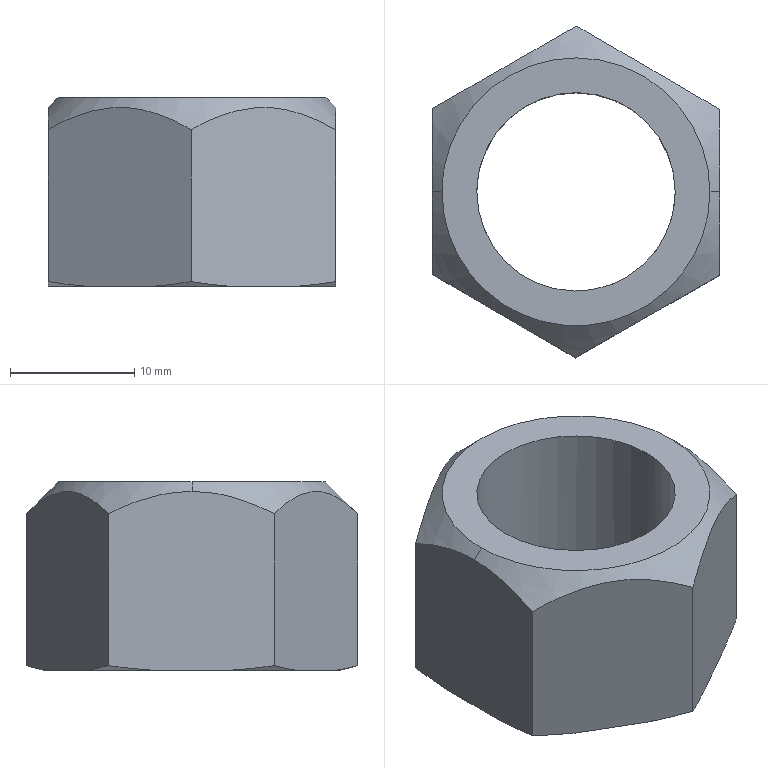Part | STEP file | GB/T6184-20001 type all-metal hex lock nut M16 | 1 solid | 20 faces | box 23.219 x 26.75 x 15.2 mm | volume 3899 mm3 | cone 10 | plane 8 | cylinder 2 | commonest cylinder face diameters 16 x2
STEP:
#1=CARTESIAN_POINT('',(-10.8,0.,15.2));
#2=VERTEX_POINT('',#1);
#3=CARTESIAN_POINT('',(10.8,0.,15.2));
#4=VERTEX_POINT('',#3);
#5=CARTESIAN_POINT('',(0.,0.,15.2));
#6=DIRECTION('',(0.,0.,-1.));
#7=AXIS2_PLACEMENT_3D('',#5,#6,$);
#8=CIRCLE('',#7,10.8);
#9=EDGE_CURVE('',#2,#4,#8,.F.);
#10=ORIENTED_EDGE('',*,*,#9,.F.);
#11=CARTESIAN_POINT('',(-11.583,0.,14.417));
#12=VERTEX_POINT('',#11);
#13=CARTESIAN_POINT('',(-353558.791,0.,-353532.791));
#14=DIRECTION('',(-0.7071,0.,-0.7071));
#15=VECTOR('',#14,1.);
#16=LINE('',#13,#15);
#17=EDGE_CURVE('',#2,#12,#16,.T.);
#18=ORIENTED_EDGE('',*,*,#17,.T.);
#19=CARTESIAN_POINT('',(-11.597,-3.411,13.912));
#20=VERTEX_POINT('',#19);
#21=CARTESIAN_POINT('',(-11.583,0.,14.417));
#22=CARTESIAN_POINT('',(-11.586,-0.8291,14.414));
#23=CARTESIAN_POINT('',(-11.59,-1.659,14.33));
#24=CARTESIAN_POINT('',(-11.593,-2.511,14.17));
#25=CARTESIAN_POINT('',(-11.597,-3.411,13.912));
#26=B_SPLINE_CURVE_WITH_KNOTS('',4,(#21,#22,#23,#24,#25),.UNSPECIFIED.,.F.,.U.,(5,5),(0.,28.825),.UNSPECIFIED.);
#27=EDGE_CURVE('',#12,#20,#26,.T.);
#28=ORIENTED_EDGE('',*,*,#27,.T.);
#29=CARTESIAN_POINT('',(-11.609,-6.642,12.625));
#30=VERTEX_POINT('',#29);
#31=CARTESIAN_POINT('',(-11.597,-3.411,13.912));
#32=CARTESIAN_POINT('',(-11.6,-4.397,13.63));
#33=CARTESIAN_POINT('',(-11.605,-5.447,13.222));
#34=CARTESIAN_POINT('',(-11.609,-6.642,12.625));
#35=B_SPLINE_CURVE_WITH_KNOTS('',3,(#31,#32,#33,#34),.UNSPECIFIED.,.F.,.U.,(4,4),(0.,23.689),.UNSPECIFIED.);
#36=EDGE_CURVE('',#20,#30,#35,.T.);
#37=ORIENTED_EDGE('',*,*,#36,.T.);
#38=CARTESIAN_POINT('',(-2.874,-11.731,13.922));
#39=VERTEX_POINT('',#38);
#40=CARTESIAN_POINT('',(-11.609,-6.642,12.625));
#41=CARTESIAN_POINT('',(-9.468,-7.889,13.864));
#42=CARTESIAN_POINT('',(-7.794,-8.865,14.408));
#43=CARTESIAN_POINT('',(-6.199,-9.794,14.622));
#44=CARTESIAN_POINT('',(-4.639,-10.703,14.5));
#45=CARTESIAN_POINT('',(-2.874,-11.731,13.922));
#46=B_SPLINE_CURVE_WITH_KNOTS('',5,(#40,#41,#42,#43,#44,#45),.UNSPECIFIED.,.F.,.U.,(6,6),(0.,81.885),.UNSPECIFIED.);
#47=EDGE_CURVE('',#30,#39,#46,.T.);
#48=ORIENTED_EDGE('',*,*,#47,.T.);
#49=CARTESIAN_POINT('',(-0.05261,-13.375,12.625));
#50=VERTEX_POINT('',#49);
#51=CARTESIAN_POINT('',(-2.874,-11.731,13.922));
#52=CARTESIAN_POINT('',(-2.013,-12.233,13.64));
#53=CARTESIAN_POINT('',(-1.097,-12.766,13.229));
#54=CARTESIAN_POINT('',(-0.05261,-13.375,12.625));
#55=B_SPLINE_CURVE_WITH_KNOTS('',3,(#51,#52,#53,#54),.UNSPECIFIED.,.F.,.U.,(4,4),(0.,23.96),.UNSPECIFIED.);
#56=EDGE_CURVE('',#39,#50,#55,.T.);
#57=ORIENTED_EDGE('',*,*,#56,.T.);
#58=CARTESIAN_POINT('',(8.723,-8.355,13.922));
#59=VERTEX_POINT('',#58);
#60=CARTESIAN_POINT('',(-0.05261,-13.375,12.625));
#61=CARTESIAN_POINT('',(2.098,-12.144,13.864));
#62=CARTESIAN_POINT('',(3.78,-11.182,14.408));
#63=CARTESIAN_POINT('',(5.382,-10.266,14.622));
#64=CARTESIAN_POINT('',(6.95,-9.369,14.5));
#65=CARTESIAN_POINT('',(8.723,-8.355,13.922));
#66=B_SPLINE_CURVE_WITH_KNOTS('',5,(#60,#61,#62,#63,#64,#65),.UNSPECIFIED.,.F.,.U.,(6,6),(0.,81.885),.UNSPECIFIED.);
#67=EDGE_CURVE('',#50,#59,#66,.T.);
#68=ORIENTED_EDGE('',*,*,#67,.T.);
#69=CARTESIAN_POINT('',(11.557,-6.733,12.625));
#70=VERTEX_POINT('',#69);
#71=CARTESIAN_POINT('',(8.723,-8.355,13.922));
#72=CARTESIAN_POINT('',(9.587,-7.86,13.64));
#73=CARTESIAN_POINT('',(10.508,-7.333,13.229));
#74=CARTESIAN_POINT('',(11.557,-6.733,12.625));
#75=B_SPLINE_CURVE_WITH_KNOTS('',3,(#71,#72,#73,#74),.UNSPECIFIED.,.F.,.U.,(4,4),(0.,23.96),.UNSPECIFIED.);
#76=EDGE_CURVE('',#59,#70,#75,.T.);
#77=ORIENTED_EDGE('',*,*,#76,.T.);
#78=CARTESIAN_POINT('',(11.583,0.,14.417));
#79=VERTEX_POINT('',#78);
#80=CARTESIAN_POINT('',(11.557,-6.733,12.625));
#81=CARTESIAN_POINT('',(11.563,-5.119,13.432));
#82=CARTESIAN_POINT('',(11.568,-3.735,13.942));
#83=CARTESIAN_POINT('',(11.574,-2.453,14.264));
#84=CARTESIAN_POINT('',(11.578,-1.227,14.422));
#85=CARTESIAN_POINT('',(11.583,0.,14.417));
#86=B_SPLINE_CURVE_WITH_KNOTS('',5,(#80,#81,#82,#83,#84,#85),.UNSPECIFIED.,.F.,.U.,(6,6),(0.,53.326),.UNSPECIFIED.);
#87=EDGE_CURVE('',#70,#79,#86,.T.);
#88=ORIENTED_EDGE('',*,*,#87,.T.);
#89=CARTESIAN_POINT('',(353558.791,0.,-353532.791));
#90=DIRECTION('',(0.7071,0.,-0.7071));
#91=VECTOR('',#90,1.);
#92=LINE('',#89,#91);
#93=EDGE_CURVE('',#4,#79,#92,.T.);
#94=ORIENTED_EDGE('',*,*,#93,.F.);
#95=EDGE_LOOP('',(#10,#18,#28,#37,#48,#57,#68,#77,#88,#94));
#96=FACE_OUTER_BOUND('',#95,.T.);
#97=CARTESIAN_POINT('',(0.,0.,15.2));
#98=DIRECTION('',(0.,0.,-1.));
#99=DIRECTION('',(1.,0.,0.));
#100=AXIS2_PLACEMENT_3D('',#97,#98,#99);
#101=CONICAL_SURFACE('',#100,10.8,0.7854);
#102=ADVANCED_FACE('',(#96),#101,.T.);
#103=CARTESIAN_POINT('',(10.8,0.,15.2));
#104=CARTESIAN_POINT('',(10.8,1.127,15.2));
#105=CARTESIAN_POINT('',(10.653,2.254,15.2));
#106=CARTESIAN_POINT('',(10.359,3.355,15.2));
#107=CARTESIAN_POINT('',(9.49,5.456,15.2));
#108=CARTESIAN_POINT('',(8.112,7.263,15.2));
#109=CARTESIAN_POINT('',(7.308,8.072,15.2));
#110=CARTESIAN_POINT('',(5.509,9.46,15.2));
#111=CARTESIAN_POINT('',(3.413,10.34,15.2));
#112=CARTESIAN_POINT('',(2.313,10.64,15.2));
#113=CARTESIAN_POINT('',(0.06074,10.947,15.2));
#114=CARTESIAN_POINT('',(-2.195,10.665,15.2));
#115=CARTESIAN_POINT('',(-3.298,10.377,15.2));
#116=CARTESIAN_POINT('',(-5.403,9.521,15.2));
#117=CARTESIAN_POINT('',(-7.218,8.152,15.2));
#118=CARTESIAN_POINT('',(-8.031,7.353,15.2));
#119=CARTESIAN_POINT('',(-9.429,5.561,15.2));
#120=CARTESIAN_POINT('',(-10.321,3.47,15.2));
#121=CARTESIAN_POINT('',(-10.627,2.372,15.2));
#122=CARTESIAN_POINT('',(-10.79,1.223,15.2));
#123=CARTESIAN_POINT('',(-10.8,0.07191,15.2));
#124=CARTESIAN_POINT('',(-10.8,0.04794,15.2));
#125=CARTESIAN_POINT('',(-10.8,0.02397,15.2));
#126=CARTESIAN_POINT('',(-10.8,0.,15.2));
#127=B_SPLINE_CURVE_WITH_KNOTS('',5,(#103,#104,#105,#106,#107,#108,#109,#110,#111,#112,#113,#114,#115,#116,#117,#118,#119,#120,#121,#122,#123,#124,#125,#126),.UNSPECIFIED.,.F.,.U.,(6,3,3,3,3,3,3,6),(0.,7.969,15.938,23.906,31.875,39.844,47.813,47.982),.UNSPECIFIED.);
#128=EDGE_CURVE('',#4,#2,#127,.T.);
#129=ORIENTED_EDGE('',*,*,#128,.T.);
#130=ORIENTED_EDGE('',*,*,#9,.T.);
#131=EDGE_LOOP('',(#129,#130));
#132=FACE_OUTER_BOUND('',#131,.T.);
#133=CARTESIAN_POINT('',(-8.,0.,15.2));
#134=VERTEX_POINT('',#133);
#135=CARTESIAN_POINT('',(8.,0.,15.2));
#136=VERTEX_POINT('',#135);
#137=CARTESIAN_POINT('',(-8.,0.,15.2));
#138=CARTESIAN_POINT('',(-8.,-0.8314,15.2));
#139=CARTESIAN_POINT('',(-7.892,-1.663,15.2));
#140=CARTESIAN_POINT('',(-7.676,-2.475,15.2));
#141=CARTESIAN_POINT('',(-7.038,-4.026,15.2));
#142=CARTESIAN_POINT('',(-6.025,-5.362,15.2));
#143=CARTESIAN_POINT('',(-5.434,-5.96,15.2));
#144=CARTESIAN_POINT('',(-4.11,-6.989,15.2));
#145=CARTESIAN_POINT('',(-2.567,-7.646,15.2));
#146=CARTESIAN_POINT('',(-1.757,-7.872,15.2));
#147=CARTESIAN_POINT('',(-0.09689,-8.107,15.2));
#148=CARTESIAN_POINT('',(1.568,-7.911,15.2));
#149=CARTESIAN_POINT('',(2.384,-7.705,15.2));
#150=CARTESIAN_POINT('',(3.942,-7.085,15.2));
#151=CARTESIAN_POINT('',(5.29,-6.088,15.2));
#152=CARTESIAN_POINT('',(5.895,-5.504,15.2));
#153=CARTESIAN_POINT('',(6.94,-4.193,15.2));
#154=CARTESIAN_POINT('',(7.615,-2.658,15.2));
#155=CARTESIAN_POINT('',(7.85,-1.851,15.2));
#156=CARTESIAN_POINT('',(7.984,-0.9842,15.2));
#157=CARTESIAN_POINT('',(7.999,-0.1147,15.2));
#158=CARTESIAN_POINT('',(8.,-0.07648,15.2));
#159=CARTESIAN_POINT('',(8.,-0.03824,15.2));
#160=CARTESIAN_POINT('',(8.,0.,15.2));
#161=B_SPLINE_CURVE_WITH_KNOTS('',5,(#137,#138,#139,#140,#141,#142,#143,#144,#145,#146,#147,#148,#149,#150,#151,#152,#153,#154,#155,#156,#157,#158,#159,#160),.UNSPECIFIED.,.F.,.U.,(6,3,3,3,3,3,3,6),(0.,5.879,11.757,17.636,23.515,29.393,35.272,35.543),.UNSPECIFIED.);
#162=EDGE_CURVE('',#134,#136,#161,.T.);
#163=ORIENTED_EDGE('',*,*,#162,.F.);
#164=CARTESIAN_POINT('',(8.,0.,15.2));
#165=CARTESIAN_POINT('',(8.,0.8314,15.2));
#166=CARTESIAN_POINT('',(7.892,1.663,15.2));
#167=CARTESIAN_POINT('',(7.676,2.475,15.2));
#168=CARTESIAN_POINT('',(7.038,4.026,15.2));
#169=CARTESIAN_POINT('',(6.025,5.362,15.2));
#170=CARTESIAN_POINT('',(5.434,5.96,15.2));
#171=CARTESIAN_POINT('',(4.11,6.989,15.2));
#172=CARTESIAN_POINT('',(2.567,7.646,15.2));
#173=CARTESIAN_POINT('',(1.757,7.872,15.2));
#174=CARTESIAN_POINT('',(0.09689,8.107,15.2));
#175=CARTESIAN_POINT('',(-1.568,7.911,15.2));
#176=CARTESIAN_POINT('',(-2.384,7.705,15.2));
#177=CARTESIAN_POINT('',(-3.942,7.085,15.2));
#178=CARTESIAN_POINT('',(-5.29,6.088,15.2));
#179=CARTESIAN_POINT('',(-5.895,5.504,15.2));
#180=CARTESIAN_POINT('',(-6.94,4.193,15.2));
#181=CARTESIAN_POINT('',(-7.615,2.658,15.2));
#182=CARTESIAN_POINT('',(-7.85,1.851,15.2));
#183=CARTESIAN_POINT('',(-7.984,0.9842,15.2));
#184=CARTESIAN_POINT('',(-7.999,0.1147,15.2));
#185=CARTESIAN_POINT('',(-8.,0.07648,15.2));
#186=CARTESIAN_POINT('',(-8.,0.03824,15.2));
#187=CARTESIAN_POINT('',(-8.,0.,15.2));
#188=B_SPLINE_CURVE_WITH_KNOTS('',5,(#164,#165,#166,#167,#168,#169,#170,#171,#172,#173,#174,#175,#176,#177,#178,#179,#180,#181,#182,#183,#184,#185,#186,#187),.UNSPECIFIED.,.F.,.U.,(6,3,3,3,3,3,3,6),(0.,5.879,11.757,17.636,23.515,29.393,35.272,35.543),.UNSPECIFIED.);
#189=EDGE_CURVE('',#136,#134,#188,.T.);
#190=ORIENTED_EDGE('',*,*,#189,.F.);
#191=EDGE_LOOP('',(#163,#190));
#192=FACE_BOUND('',#191,.T.);
#193=CARTESIAN_POINT('',(23.166,-0.09113,15.2));
#194=DIRECTION('',(0.,0.,-1.));
#195=DIRECTION('',(-1.,0.,0.));
#196=AXIS2_PLACEMENT_3D('',#193,#194,#195);
#197=PLANE('',#196);
#198=ADVANCED_FACE('',(#132,#192),#197,.F.);
#199=ORIENTED_EDGE('',*,*,#17,.F.);
#200=ORIENTED_EDGE('',*,*,#128,.F.);
#201=ORIENTED_EDGE('',*,*,#93,.T.);
#202=CARTESIAN_POINT('',(11.597,3.411,13.912));
#203=VERTEX_POINT('',#202);
#204=CARTESIAN_POINT('',(11.583,0.,14.417));
#205=CARTESIAN_POINT('',(11.586,0.8291,14.414));
#206=CARTESIAN_POINT('',(11.59,1.659,14.33));
#207=CARTESIAN_POINT('',(11.593,2.511,14.17));
#208=CARTESIAN_POINT('',(11.597,3.411,13.912));
#209=B_SPLINE_CURVE_WITH_KNOTS('',4,(#204,#205,#206,#207,#208),.UNSPECIFIED.,.F.,.U.,(5,5),(0.,28.825),.UNSPECIFIED.);
#210=EDGE_CURVE('',#79,#203,#209,.T.);
#211=ORIENTED_EDGE('',*,*,#210,.T.);
#212=CARTESIAN_POINT('',(11.609,6.642,12.625));
#213=VERTEX_POINT('',#212);
#214=CARTESIAN_POINT('',(11.597,3.411,13.912));
#215=CARTESIAN_POINT('',(11.6,4.397,13.63));
#216=CARTESIAN_POINT('',(11.605,5.447,13.222));
#217=CARTESIAN_POINT('',(11.609,6.642,12.625));
#218=B_SPLINE_CURVE_WITH_KNOTS('',3,(#214,#215,#216,#217),.UNSPECIFIED.,.F.,.U.,(4,4),(0.,23.689),.UNSPECIFIED.);
#219=EDGE_CURVE('',#203,#213,#218,.T.);
#220=ORIENTED_EDGE('',*,*,#219,.T.);
#221=CARTESIAN_POINT('',(2.874,11.731,13.922));
#222=VERTEX_POINT('',#221);
#223=CARTESIAN_POINT('',(11.609,6.642,12.625));
#224=CARTESIAN_POINT('',(9.468,7.889,13.864));
#225=CARTESIAN_POINT('',(7.794,8.865,14.408));
#226=CARTESIAN_POINT('',(6.199,9.794,14.622));
#227=CARTESIAN_POINT('',(4.639,10.703,14.5));
#228=CARTESIAN_POINT('',(2.874,11.731,13.922));
#229=B_SPLINE_CURVE_WITH_KNOTS('',5,(#223,#224,#225,#226,#227,#228),.UNSPECIFIED.,.F.,.U.,(6,6),(0.,81.885),.UNSPECIFIED.);
#230=EDGE_CURVE('',#213,#222,#229,.T.);
#231=ORIENTED_EDGE('',*,*,#230,.T.);
#232=CARTESIAN_POINT('',(0.05261,13.375,12.625));
#233=VERTEX_POINT('',#232);
#234=CARTESIAN_POINT('',(2.874,11.731,13.922));
#235=CARTESIAN_POINT('',(2.013,12.233,13.64));
#236=CARTESIAN_POINT('',(1.097,12.766,13.229));
#237=CARTESIAN_POINT('',(0.05261,13.375,12.625));
#238=B_SPLINE_CURVE_WITH_KNOTS('',3,(#234,#235,#236,#237),.UNSPECIFIED.,.F.,.U.,(4,4),(0.,23.96),.UNSPECIFIED.);
#239=EDGE_CURVE('',#222,#233,#238,.T.);
#240=ORIENTED_EDGE('',*,*,#239,.T.);
#241=CARTESIAN_POINT('',(-8.722,8.355,13.922));
#242=VERTEX_POINT('',#241);
#243=CARTESIAN_POINT('',(0.05261,13.375,12.625));
#244=CARTESIAN_POINT('',(-2.098,12.144,13.864));
#245=CARTESIAN_POINT('',(-3.78,11.182,14.408));
#246=CARTESIAN_POINT('',(-5.382,10.266,14.622));
#247=CARTESIAN_POINT('',(-6.95,9.369,14.5));
#248=CARTESIAN_POINT('',(-8.723,8.355,13.922));
#249=B_SPLINE_CURVE_WITH_KNOTS('',5,(#243,#244,#245,#246,#247,#248),.UNSPECIFIED.,.F.,.U.,(6,6),(0.,81.885),.UNSPECIFIED.);
#250=EDGE_CURVE('',#233,#242,#249,.T.);
#251=ORIENTED_EDGE('',*,*,#250,.T.);
#252=CARTESIAN_POINT('',(-11.557,6.733,12.625));
#253=VERTEX_POINT('',#252);
#254=CARTESIAN_POINT('',(-8.723,8.355,13.922));
#255=CARTESIAN_POINT('',(-9.587,7.86,13.64));
#256=CARTESIAN_POINT('',(-10.508,7.333,13.229));
#257=CARTESIAN_POINT('',(-11.557,6.733,12.625));
#258=B_SPLINE_CURVE_WITH_KNOTS('',3,(#254,#255,#256,#257),.UNSPECIFIED.,.F.,.U.,(4,4),(0.,23.96),.UNSPECIFIED.);
#259=EDGE_CURVE('',#242,#253,#258,.T.);
#260=ORIENTED_EDGE('',*,*,#259,.T.);
#261=CARTESIAN_POINT('',(-11.557,6.733,12.625));
#262=CARTESIAN_POINT('',(-11.563,5.119,13.432));
#263=CARTESIAN_POINT('',(-11.568,3.735,13.942));
#264=CARTESIAN_POINT('',(-11.574,2.453,14.264));
#265=CARTESIAN_POINT('',(-11.578,1.227,14.422));
#266=CARTESIAN_POINT('',(-11.583,0.,14.417));
#267=B_SPLINE_CURVE_WITH_KNOTS('',5,(#261,#262,#263,#264,#265,#266),.UNSPECIFIED.,.F.,.U.,(6,6),(0.,53.326),.UNSPECIFIED.);
#268=EDGE_CURVE('',#253,#12,#267,.T.);
#269=ORIENTED_EDGE('',*,*,#268,.T.);
#270=EDGE_LOOP('',(#199,#200,#201,#211,#220,#231,#240,#251,#260,#269));
#271=FACE_OUTER_BOUND('',#270,.T.);
#272=CARTESIAN_POINT('',(0.,0.,15.2));
#273=DIRECTION('',(0.,0.,-1.));
#274=DIRECTION('',(-1.,0.,0.));
#275=AXIS2_PLACEMENT_3D('',#272,#273,#274);
#276=CONICAL_SURFACE('',#275,10.8,0.7854);
#277=ADVANCED_FACE('',(#271),#276,.T.);
#278=ORIENTED_EDGE('',*,*,#268,.F.);
#279=CARTESIAN_POINT('',(-11.557,6.733,0.3684));
#280=VERTEX_POINT('',#279);
#281=CARTESIAN_POINT('',(-11.557,6.733,6.497));
#282=DIRECTION('',(0.,0.,-1.));
#283=VECTOR('',#282,1.);
#284=LINE('',#281,#283);
#285=EDGE_CURVE('',#253,#280,#284,.T.);
#286=ORIENTED_EDGE('',*,*,#285,.T.);
#287=CARTESIAN_POINT('',(-11.571,3.181,0.000000001));
#288=VERTEX_POINT('',#287);
#289=CARTESIAN_POINT('',(-11.571,3.181,0.000000001));
#290=CARTESIAN_POINT('',(-11.568,3.752,0.03994));
#291=CARTESIAN_POINT('',(-11.566,4.322,0.08839));
#292=CARTESIAN_POINT('',(-11.564,4.89,0.1444));
#293=CARTESIAN_POINT('',(-11.561,5.6,0.2236));
#294=CARTESIAN_POINT('',(-11.558,6.309,0.3127));
#295=CARTESIAN_POINT('',(-11.558,6.45,0.3309));
#296=CARTESIAN_POINT('',(-11.557,6.592,0.3495));
#297=CARTESIAN_POINT('',(-11.557,6.733,0.3684));
#298=B_SPLINE_CURVE_WITH_KNOTS('',5,(#289,#290,#291,#292,#293,#294,#295,#296,#297),.UNSPECIFIED.,.F.,.U.,(6,3,6),(0.,4.044,5.053),.UNSPECIFIED.);
#299=EDGE_CURVE('',#288,#280,#298,.T.);
#300=ORIENTED_EDGE('',*,*,#299,.F.);
#301=CARTESIAN_POINT('',(-11.595,-3.09,0.000000001));
#302=VERTEX_POINT('',#301);
#303=CARTESIAN_POINT('',(-11.583,0.04556,0.000000001));
#304=DIRECTION('',(-0.003934,-1.,0.));
#305=VECTOR('',#304,1.);
#306=LINE('',#303,#305);
#307=EDGE_CURVE('',#288,#302,#306,.T.);
#308=ORIENTED_EDGE('',*,*,#307,.T.);
#309=CARTESIAN_POINT('',(-11.609,-6.642,0.3684));
#310=VERTEX_POINT('',#309);
#311=CARTESIAN_POINT('',(-11.609,-6.642,0.3684));
#312=CARTESIAN_POINT('',(-11.607,-5.934,0.2736));
#313=CARTESIAN_POINT('',(-11.604,-5.225,0.188));
#314=CARTESIAN_POINT('',(-11.601,-4.514,0.113));
#315=CARTESIAN_POINT('',(-11.598,-3.803,0.04991));
#316=CARTESIAN_POINT('',(-11.595,-3.09,0.000000001));
#317=B_SPLINE_CURVE_WITH_KNOTS('',5,(#311,#312,#313,#314,#315,#316),.UNSPECIFIED.,.F.,.U.,(6,6),(0.,5.051),.UNSPECIFIED.);
#318=EDGE_CURVE('',#310,#302,#317,.T.);
#319=ORIENTED_EDGE('',*,*,#318,.F.);
#320=CARTESIAN_POINT('',(-11.609,-6.642,6.497));
#321=DIRECTION('',(0.,0.,-1.));
#322=VECTOR('',#321,1.);
#323=LINE('',#320,#322);
#324=EDGE_CURVE('',#30,#310,#323,.T.);
#325=ORIENTED_EDGE('',*,*,#324,.F.);
#326=ORIENTED_EDGE('',*,*,#36,.F.);
#327=ORIENTED_EDGE('',*,*,#27,.F.);
#328=EDGE_LOOP('',(#278,#286,#300,#308,#319,#325,#326,#327));
#329=FACE_OUTER_BOUND('',#328,.T.);
#330=CARTESIAN_POINT('',(-11.557,6.733,15.2));
#331=DIRECTION('',(1.,-0.003934,0.));
#332=DIRECTION('',(0.003934,1.,0.));
#333=AXIS2_PLACEMENT_3D('',#330,#331,#332);
#334=PLANE('',#333);
#335=ADVANCED_FACE('',(#329),#334,.F.);
#336=ORIENTED_EDGE('',*,*,#56,.F.);
#337=ORIENTED_EDGE('',*,*,#47,.F.);
#338=ORIENTED_EDGE('',*,*,#324,.T.);
#339=CARTESIAN_POINT('',(-8.54,-8.43,0.000000001));
#340=VERTEX_POINT('',#339);
#341=CARTESIAN_POINT('',(-8.54,-8.43,0.000000001));
#342=CARTESIAN_POINT('',(-9.156,-8.071,0.04992));
#343=CARTESIAN_POINT('',(-9.771,-7.713,0.1131));
#344=CARTESIAN_POINT('',(-10.386,-7.355,0.1881));
#345=CARTESIAN_POINT('',(-10.998,-6.998,0.2737));
#346=CARTESIAN_POINT('',(-11.609,-6.642,0.3684));
#347=B_SPLINE_CURVE_WITH_KNOTS('',5,(#341,#342,#343,#344,#345,#346),.UNSPECIFIED.,.F.,.U.,(6,6),(0.,5.051),.UNSPECIFIED.);
#348=EDGE_CURVE('',#340,#310,#347,.T.);
#349=ORIENTED_EDGE('',*,*,#348,.F.);
#350=CARTESIAN_POINT('',(-3.122,-11.587,0.000000001));
#351=VERTEX_POINT('',#350);
#352=CARTESIAN_POINT('',(-5.831,-10.008,0.000000001));
#353=DIRECTION('',(0.8641,-0.5034,0.));
#354=VECTOR('',#353,1.);
#355=LINE('',#352,#354);
#356=EDGE_CURVE('',#340,#351,#355,.T.);
#357=ORIENTED_EDGE('',*,*,#356,.T.);
#358=CARTESIAN_POINT('',(-0.05261,-13.375,0.3684));
#359=VERTEX_POINT('',#358);
#360=CARTESIAN_POINT('',(-0.05261,-13.375,0.3684));
#361=CARTESIAN_POINT('',(-0.6642,-13.019,0.2736));
#362=CARTESIAN_POINT('',(-1.277,-12.662,0.188));
#363=CARTESIAN_POINT('',(-1.891,-12.304,0.113));
#364=CARTESIAN_POINT('',(-2.506,-11.946,0.04992));
#365=CARTESIAN_POINT('',(-3.122,-11.587,0.000000001));
#366=B_SPLINE_CURVE_WITH_KNOTS('',5,(#360,#361,#362,#363,#364,#365),.UNSPECIFIED.,.F.,.U.,(6,6),(0.,5.051),.UNSPECIFIED.);
#367=EDGE_CURVE('',#359,#351,#366,.T.);
#368=ORIENTED_EDGE('',*,*,#367,.F.);
#369=CARTESIAN_POINT('',(-0.05261,-13.375,6.497));
#370=DIRECTION('',(0.,0.,-1.));
#371=VECTOR('',#370,1.);
#372=LINE('',#369,#371);
#373=EDGE_CURVE('',#50,#359,#372,.T.);
#374=ORIENTED_EDGE('',*,*,#373,.F.);
#375=EDGE_LOOP('',(#336,#337,#338,#349,#357,#368,#374));
#376=FACE_OUTER_BOUND('',#375,.T.);
#377=CARTESIAN_POINT('',(-11.609,-6.642,15.2));
#378=DIRECTION('',(0.5034,0.8641,0.));
#379=DIRECTION('',(-0.8641,0.5034,0.));
#380=AXIS2_PLACEMENT_3D('',#377,#378,#379);
#381=PLANE('',#380);
#382=ADVANCED_FACE('',(#376),#381,.F.);
#383=ORIENTED_EDGE('',*,*,#76,.F.);
#384=ORIENTED_EDGE('',*,*,#67,.F.);
#385=ORIENTED_EDGE('',*,*,#373,.T.);
#386=CARTESIAN_POINT('',(3.03,-11.611,0.000000001));
#387=VERTEX_POINT('',#386);
#388=CARTESIAN_POINT('',(3.03,-11.611,0.000000001));
#389=CARTESIAN_POINT('',(2.412,-11.965,0.04992));
#390=CARTESIAN_POINT('',(1.794,-12.319,0.1131));
#391=CARTESIAN_POINT('',(1.177,-12.672,0.1881));
#392=CARTESIAN_POINT('',(0.5613,-13.024,0.2737));
#393=CARTESIAN_POINT('',(-0.05261,-13.375,0.3684));
#394=B_SPLINE_CURVE_WITH_KNOTS('',5,(#388,#389,#390,#391,#392,#393),.UNSPECIFIED.,.F.,.U.,(6,6),(0.,5.051),.UNSPECIFIED.);
#395=EDGE_CURVE('',#387,#359,#394,.T.);
#396=ORIENTED_EDGE('',*,*,#395,.F.);
#397=CARTESIAN_POINT('',(8.474,-8.497,0.000000001));
#398=VERTEX_POINT('',#397);
#399=CARTESIAN_POINT('',(5.752,-10.054,0.000000001));
#400=DIRECTION('',(0.868,0.4966,0.));
#401=VECTOR('',#400,1.);
#402=LINE('',#399,#401);
#403=EDGE_CURVE('',#387,#398,#402,.T.);
#404=ORIENTED_EDGE('',*,*,#403,.T.);
#405=CARTESIAN_POINT('',(11.557,-6.733,0.3684));
#406=VERTEX_POINT('',#405);
#407=CARTESIAN_POINT('',(11.557,-6.733,0.3684));
#408=CARTESIAN_POINT('',(10.942,-7.084,0.2736));
#409=CARTESIAN_POINT('',(10.327,-7.437,0.188));
#410=CARTESIAN_POINT('',(9.71,-7.789,0.113));
#411=CARTESIAN_POINT('',(9.093,-8.143,0.04992));
#412=CARTESIAN_POINT('',(8.474,-8.497,0.000000001));
#413=B_SPLINE_CURVE_WITH_KNOTS('',5,(#407,#408,#409,#410,#411,#412),.UNSPECIFIED.,.F.,.U.,(6,6),(0.,5.051),.UNSPECIFIED.);
#414=EDGE_CURVE('',#406,#398,#413,.T.);
#415=ORIENTED_EDGE('',*,*,#414,.F.);
#416=CARTESIAN_POINT('',(11.557,-6.733,6.497));
#417=DIRECTION('',(0.,0.,-1.));
#418=VECTOR('',#417,1.);
#419=LINE('',#416,#418);
#420=EDGE_CURVE('',#70,#406,#419,.T.);
#421=ORIENTED_EDGE('',*,*,#420,.F.);
#422=EDGE_LOOP('',(#383,#384,#385,#396,#404,#415,#421));
#423=FACE_OUTER_BOUND('',#422,.T.);
#424=CARTESIAN_POINT('',(-0.05261,-13.375,15.2));
#425=DIRECTION('',(-0.4966,0.868,0.));
#426=DIRECTION('',(-0.868,-0.4966,0.));
#427=AXIS2_PLACEMENT_3D('',#424,#425,#426);
#428=PLANE('',#427);
#429=ADVANCED_FACE('',(#423),#428,.F.);
#430=ORIENTED_EDGE('',*,*,#87,.F.);
#431=ORIENTED_EDGE('',*,*,#420,.T.);
#432=CARTESIAN_POINT('',(11.571,-3.181,0.000000001));
#433=VERTEX_POINT('',#432);
#434=CARTESIAN_POINT('',(11.571,-3.181,0.000000001));
#435=CARTESIAN_POINT('',(11.568,-3.752,0.03994));
#436=CARTESIAN_POINT('',(11.566,-4.322,0.08839));
#437=CARTESIAN_POINT('',(11.564,-4.89,0.1444));
#438=CARTESIAN_POINT('',(11.561,-5.6,0.2236));
#439=CARTESIAN_POINT('',(11.558,-6.309,0.3127));
#440=CARTESIAN_POINT('',(11.558,-6.45,0.3309));
#441=CARTESIAN_POINT('',(11.557,-6.592,0.3495));
#442=CARTESIAN_POINT('',(11.557,-6.733,0.3684));
#443=B_SPLINE_CURVE_WITH_KNOTS('',5,(#434,#435,#436,#437,#438,#439,#440,#441,#442),.UNSPECIFIED.,.F.,.U.,(6,3,6),(0.,4.044,5.053),.UNSPECIFIED.);
#444=EDGE_CURVE('',#433,#406,#443,.T.);
#445=ORIENTED_EDGE('',*,*,#444,.F.);
#446=CARTESIAN_POINT('',(11.595,3.09,0.000000001));
#447=VERTEX_POINT('',#446);
#448=CARTESIAN_POINT('',(11.583,-0.04556,0.000000001));
#449=DIRECTION('',(0.003934,1.,0.));
#450=VECTOR('',#449,1.);
#451=LINE('',#448,#450);
#452=EDGE_CURVE('',#433,#447,#451,.T.);
#453=ORIENTED_EDGE('',*,*,#452,.T.);
#454=CARTESIAN_POINT('',(11.609,6.642,0.3684));
#455=VERTEX_POINT('',#454);
#456=CARTESIAN_POINT('',(11.609,6.642,0.3684));
#457=CARTESIAN_POINT('',(11.607,5.934,0.2736));
#458=CARTESIAN_POINT('',(11.604,5.225,0.188));
#459=CARTESIAN_POINT('',(11.601,4.514,0.113));
#460=CARTESIAN_POINT('',(11.598,3.803,0.04991));
#461=CARTESIAN_POINT('',(11.595,3.09,0.000000001));
#462=B_SPLINE_CURVE_WITH_KNOTS('',5,(#456,#457,#458,#459,#460,#461),.UNSPECIFIED.,.F.,.U.,(6,6),(0.,5.051),.UNSPECIFIED.);
#463=EDGE_CURVE('',#455,#447,#462,.T.);
#464=ORIENTED_EDGE('',*,*,#463,.F.);
#465=CARTESIAN_POINT('',(11.609,6.642,6.497));
#466=DIRECTION('',(0.,0.,-1.));
#467=VECTOR('',#466,1.);
#468=LINE('',#465,#467);
#469=EDGE_CURVE('',#213,#455,#468,.T.);
#470=ORIENTED_EDGE('',*,*,#469,.F.);
#471=ORIENTED_EDGE('',*,*,#219,.F.);
#472=ORIENTED_EDGE('',*,*,#210,.F.);
#473=EDGE_LOOP('',(#430,#431,#445,#453,#464,#470,#471,#472));
#474=FACE_OUTER_BOUND('',#473,.T.);
#475=CARTESIAN_POINT('',(11.557,-6.733,15.2));
#476=DIRECTION('',(-1.,0.003934,0.));
#477=DIRECTION('',(-0.003934,-1.,0.));
#478=AXIS2_PLACEMENT_3D('',#475,#476,#477);
#479=PLANE('',#478);
#480=ADVANCED_FACE('',(#474),#479,.F.);
#481=ORIENTED_EDGE('',*,*,#162,.T.);
#482=CARTESIAN_POINT('',(8.,0.,1.031));
#483=VERTEX_POINT('',#482);
#484=CARTESIAN_POINT('',(8.,0.,15.2));
#485=DIRECTION('',(0.,0.,-1.));
#486=VECTOR('',#485,1.);
#487=LINE('',#484,#486);
#488=EDGE_CURVE('',#136,#483,#487,.T.);
#489=ORIENTED_EDGE('',*,*,#488,.T.);
#490=CARTESIAN_POINT('',(-8.,0.,1.031));
#491=VERTEX_POINT('',#490);
#492=CARTESIAN_POINT('',(8.,0.,1.031));
#493=CARTESIAN_POINT('',(8.,-1.257,1.031));
#494=CARTESIAN_POINT('',(7.753,-2.513,1.031));
#495=CARTESIAN_POINT('',(7.26,-3.705,1.031));
#496=CARTESIAN_POINT('',(5.831,-5.831,1.031));
#497=CARTESIAN_POINT('',(3.705,-7.26,1.031));
#498=CARTESIAN_POINT('',(2.513,-7.753,1.031));
#499=CARTESIAN_POINT('',(0.,-8.247,1.031));
#500=CARTESIAN_POINT('',(-2.513,-7.753,1.031));
#501=CARTESIAN_POINT('',(-3.705,-7.26,1.031));
#502=CARTESIAN_POINT('',(-5.831,-5.831,1.031));
#503=CARTESIAN_POINT('',(-7.26,-3.705,1.031));
#504=CARTESIAN_POINT('',(-7.753,-2.513,1.031));
#505=CARTESIAN_POINT('',(-8.,-1.257,1.031));
#506=CARTESIAN_POINT('',(-8.,0.,1.031));
#507=B_SPLINE_CURVE_WITH_KNOTS('',5,(#492,#493,#494,#495,#496,#497,#498,#499,#500,#501,#502,#503,#504,#505,#506),.UNSPECIFIED.,.F.,.U.,(6,3,3,3,6),(-12.566,-6.283,0.,6.283,12.566),.UNSPECIFIED.);
#508=EDGE_CURVE('',#483,#491,#507,.T.);
#509=ORIENTED_EDGE('',*,*,#508,.T.);
#510=CARTESIAN_POINT('',(-8.,0.,15.2));
#511=DIRECTION('',(0.,0.,-1.));
#512=VECTOR('',#511,1.);
#513=LINE('',#510,#512);
#514=EDGE_CURVE('',#134,#491,#513,.T.);
#515=ORIENTED_EDGE('',*,*,#514,.F.);
#516=EDGE_LOOP('',(#481,#489,#509,#515));
#517=FACE_OUTER_BOUND('',#516,.T.);
#518=CARTESIAN_POINT('',(0.,0.,15.2));
#519=DIRECTION('',(0.,0.,-1.));
#520=DIRECTION('',(1.,0.,0.));
#521=AXIS2_PLACEMENT_3D('',#518,#519,#520);
#522=CYLINDRICAL_SURFACE('',#521,8.);
#523=ADVANCED_FACE('',(#517),#522,.F.);
#524=ORIENTED_EDGE('',*,*,#488,.F.);
#525=ORIENTED_EDGE('',*,*,#189,.T.);
#526=ORIENTED_EDGE('',*,*,#514,.T.);
#527=CARTESIAN_POINT('',(0.,0.,1.031));
#528=DIRECTION('',(0.,0.,-1.));
#529=AXIS2_PLACEMENT_3D('',#527,#528,$);
#530=CIRCLE('',#529,8.);
#531=EDGE_CURVE('',#491,#483,#530,.T.);
#532=ORIENTED_EDGE('',*,*,#531,.T.);
#533=EDGE_LOOP('',(#524,#525,#526,#532));
#534=FACE_OUTER_BOUND('',#533,.T.);
#535=CARTESIAN_POINT('',(0.,0.,15.2));
#536=DIRECTION('',(0.,0.,-1.));
#537=DIRECTION('',(-1.,0.,0.));
#538=AXIS2_PLACEMENT_3D('',#535,#536,#537);
#539=CYLINDRICAL_SURFACE('',#538,8.);
#540=ADVANCED_FACE('',(#534),#539,.F.);
#541=ORIENTED_EDGE('',*,*,#239,.F.);
#542=ORIENTED_EDGE('',*,*,#230,.F.);
#543=ORIENTED_EDGE('',*,*,#469,.T.);
#544=CARTESIAN_POINT('',(8.54,8.43,0.000000001));
#545=VERTEX_POINT('',#544);
#546=CARTESIAN_POINT('',(8.54,8.43,0.000000001));
#547=CARTESIAN_POINT('',(9.156,8.071,0.04992));
#548=CARTESIAN_POINT('',(9.771,7.713,0.1131));
#549=CARTESIAN_POINT('',(10.386,7.355,0.1881));
#550=CARTESIAN_POINT('',(10.998,6.998,0.2737));
#551=CARTESIAN_POINT('',(11.609,6.642,0.3684));
#552=B_SPLINE_CURVE_WITH_KNOTS('',5,(#546,#547,#548,#549,#550,#551),.UNSPECIFIED.,.F.,.U.,(6,6),(0.,5.051),.UNSPECIFIED.);
#553=EDGE_CURVE('',#545,#455,#552,.T.);
#554=ORIENTED_EDGE('',*,*,#553,.F.);
#555=CARTESIAN_POINT('',(3.122,11.587,0.000000001));
#556=VERTEX_POINT('',#555);
#557=CARTESIAN_POINT('',(5.831,10.008,0.000000001));
#558=DIRECTION('',(-0.8641,0.5034,0.));
#559=VECTOR('',#558,1.);
#560=LINE('',#557,#559);
#561=EDGE_CURVE('',#545,#556,#560,.T.);
#562=ORIENTED_EDGE('',*,*,#561,.T.);
#563=CARTESIAN_POINT('',(0.05261,13.375,0.3684));
#564=VERTEX_POINT('',#563);
#565=CARTESIAN_POINT('',(0.05261,13.375,0.3684));
#566=CARTESIAN_POINT('',(0.6642,13.019,0.2736));
#567=CARTESIAN_POINT('',(1.277,12.662,0.188));
#568=CARTESIAN_POINT('',(1.891,12.304,0.113));
#569=CARTESIAN_POINT('',(2.506,11.946,0.04992));
#570=CARTESIAN_POINT('',(3.122,11.587,0.000000001));
#571=B_SPLINE_CURVE_WITH_KNOTS('',5,(#565,#566,#567,#568,#569,#570),.UNSPECIFIED.,.F.,.U.,(6,6),(0.,5.051),.UNSPECIFIED.);
#572=EDGE_CURVE('',#564,#556,#571,.T.);
#573=ORIENTED_EDGE('',*,*,#572,.F.);
#574=CARTESIAN_POINT('',(0.05261,13.375,6.497));
#575=DIRECTION('',(0.,0.,-1.));
#576=VECTOR('',#575,1.);
#577=LINE('',#574,#576);
#578=EDGE_CURVE('',#233,#564,#577,.T.);
#579=ORIENTED_EDGE('',*,*,#578,.F.);
#580=EDGE_LOOP('',(#541,#542,#543,#554,#562,#573,#579));
#581=FACE_OUTER_BOUND('',#580,.T.);
#582=CARTESIAN_POINT('',(11.609,6.642,15.2));
#583=DIRECTION('',(-0.5034,-0.8641,0.));
#584=DIRECTION('',(0.8641,-0.5034,0.));
#585=AXIS2_PLACEMENT_3D('',#582,#583,#584);
#586=PLANE('',#585);
#587=ADVANCED_FACE('',(#581),#586,.F.);
#588=ORIENTED_EDGE('',*,*,#259,.F.);
#589=ORIENTED_EDGE('',*,*,#250,.F.);
#590=ORIENTED_EDGE('',*,*,#578,.T.);
#591=CARTESIAN_POINT('',(-3.03,11.611,0.000000001));
#592=VERTEX_POINT('',#591);
#593=CARTESIAN_POINT('',(-3.03,11.611,0.000000001));
#594=CARTESIAN_POINT('',(-2.412,11.965,0.04992));
#595=CARTESIAN_POINT('',(-1.794,12.319,0.1131));
#596=CARTESIAN_POINT('',(-1.177,12.672,0.1881));
#597=CARTESIAN_POINT('',(-0.5613,13.024,0.2737));
#598=CARTESIAN_POINT('',(0.05261,13.375,0.3684));
#599=B_SPLINE_CURVE_WITH_KNOTS('',5,(#593,#594,#595,#596,#597,#598),.UNSPECIFIED.,.F.,.U.,(6,6),(0.,5.051),.UNSPECIFIED.);
#600=EDGE_CURVE('',#592,#564,#599,.T.);
#601=ORIENTED_EDGE('',*,*,#600,.F.);
#602=CARTESIAN_POINT('',(-8.474,8.497,0.000000001));
#603=VERTEX_POINT('',#602);
#604=CARTESIAN_POINT('',(-5.752,10.054,0.000000001));
#605=DIRECTION('',(-0.868,-0.4966,0.));
#606=VECTOR('',#605,1.);
#607=LINE('',#604,#606);
#608=EDGE_CURVE('',#592,#603,#607,.T.);
#609=ORIENTED_EDGE('',*,*,#608,.T.);
#610=CARTESIAN_POINT('',(-11.557,6.733,0.3684));
#611=CARTESIAN_POINT('',(-10.942,7.084,0.2736));
#612=CARTESIAN_POINT('',(-10.327,7.437,0.188));
#613=CARTESIAN_POINT('',(-9.71,7.789,0.113));
#614=CARTESIAN_POINT('',(-9.093,8.143,0.04992));
#615=CARTESIAN_POINT('',(-8.474,8.497,0.000000001));
#616=B_SPLINE_CURVE_WITH_KNOTS('',5,(#610,#611,#612,#613,#614,#615),.UNSPECIFIED.,.F.,.U.,(6,6),(0.,5.051),.UNSPECIFIED.);
#617=EDGE_CURVE('',#280,#603,#616,.T.);
#618=ORIENTED_EDGE('',*,*,#617,.F.);
#619=ORIENTED_EDGE('',*,*,#285,.F.);
#620=EDGE_LOOP('',(#588,#589,#590,#601,#609,#618,#619));
#621=FACE_OUTER_BOUND('',#620,.T.);
#622=CARTESIAN_POINT('',(0.05261,13.375,15.2));
#623=DIRECTION('',(0.4966,-0.868,0.));
#624=DIRECTION('',(0.868,0.4966,0.));
#625=AXIS2_PLACEMENT_3D('',#622,#623,#624);
#626=PLANE('',#625);
#627=ADVANCED_FACE('',(#621),#626,.F.);
#628=ORIENTED_EDGE('',*,*,#617,.T.);
#629=CARTESIAN_POINT('',(0.,0.,0.));
#630=DIRECTION('',(0.,0.,1.));
#631=AXIS2_PLACEMENT_3D('',#629,#630,$);
#632=CIRCLE('',#631,12.);
#633=EDGE_CURVE('',#288,#603,#632,.F.);
#634=ORIENTED_EDGE('',*,*,#633,.F.);
#635=ORIENTED_EDGE('',*,*,#299,.T.);
#636=EDGE_LOOP('',(#628,#634,#635));
#637=FACE_OUTER_BOUND('',#636,.T.);
#638=CARTESIAN_POINT('',(0.,0.,0.));
#639=DIRECTION('',(0.,0.,1.));
#640=DIRECTION('',(1.,0.,0.));
#641=AXIS2_PLACEMENT_3D('',#638,#639,#640);
#642=CONICAL_SURFACE('',#641,12.,1.309);
#643=ADVANCED_FACE('',(#637),#642,.T.);
#644=ORIENTED_EDGE('',*,*,#307,.F.);
#645=ORIENTED_EDGE('',*,*,#633,.T.);
#646=ORIENTED_EDGE('',*,*,#608,.F.);
#647=CARTESIAN_POINT('',(-0.000000001,-0.000000036,0.));
#648=DIRECTION('',(0.,0.,-1.));
#649=AXIS2_PLACEMENT_3D('',#647,#648,$);
#650=CIRCLE('',#649,12.);
#651=EDGE_CURVE('',#592,#556,#650,.T.);
#652=ORIENTED_EDGE('',*,*,#651,.T.);
#653=ORIENTED_EDGE('',*,*,#561,.F.);
#654=CARTESIAN_POINT('',(-0.000000015,-0.00000001,0.));
#655=DIRECTION('',(0.,0.,-1.));
#656=AXIS2_PLACEMENT_3D('',#654,#655,$);
#657=CIRCLE('',#656,12.);
#658=EDGE_CURVE('',#545,#447,#657,.T.);
#659=ORIENTED_EDGE('',*,*,#658,.T.);
#660=ORIENTED_EDGE('',*,*,#452,.F.);
#661=CARTESIAN_POINT('',(0.000000007,-0.000000005,0.));
#662=DIRECTION('',(0.,0.,-1.));
#663=AXIS2_PLACEMENT_3D('',#661,#662,$);
#664=CIRCLE('',#663,12.);
#665=EDGE_CURVE('',#433,#398,#664,.T.);
#666=ORIENTED_EDGE('',*,*,#665,.T.);
#667=ORIENTED_EDGE('',*,*,#403,.F.);
#668=CARTESIAN_POINT('',(-0.000000003,0.000000002,0.));
#669=DIRECTION('',(0.,0.,-1.));
#670=AXIS2_PLACEMENT_3D('',#668,#669,$);
#671=CIRCLE('',#670,12.);
#672=EDGE_CURVE('',#387,#351,#671,.T.);
#673=ORIENTED_EDGE('',*,*,#672,.T.);
#674=ORIENTED_EDGE('',*,*,#356,.F.);
#675=CARTESIAN_POINT('',(0.000000016,0.000000009,0.));
#676=DIRECTION('',(0.,0.,-1.));
#677=AXIS2_PLACEMENT_3D('',#675,#676,$);
#678=CIRCLE('',#677,12.);
#679=EDGE_CURVE('',#340,#302,#678,.T.);
#680=ORIENTED_EDGE('',*,*,#679,.T.);
#681=EDGE_LOOP('',(#644,#645,#646,#652,#653,#659,#660,#666,#667,#673,#674,#680));
#682=FACE_OUTER_BOUND('',#681,.T.);
#683=CARTESIAN_POINT('',(-9.031,0.,0.));
#684=VERTEX_POINT('',#683);
#685=CARTESIAN_POINT('',(9.031,0.,0.));
#686=VERTEX_POINT('',#685);
#687=CARTESIAN_POINT('',(-9.031,0.,0.));
#688=CARTESIAN_POINT('',(-9.031,-0.8833,0.));
#689=CARTESIAN_POINT('',(-8.923,-1.767,0.));
#690=CARTESIAN_POINT('',(-8.707,-2.632,0.));
#691=CARTESIAN_POINT('',(-8.068,-4.293,0.));
#692=CARTESIAN_POINT('',(-7.047,-5.752,0.));
#693=CARTESIAN_POINT('',(-6.45,-6.414,0.));
#694=CARTESIAN_POINT('',(-5.105,-7.58,0.));
#695=CARTESIAN_POINT('',(-3.519,-8.388,0.));
#696=CARTESIAN_POINT('',(-2.68,-8.692,0.));
#697=CARTESIAN_POINT('',(-0.9453,-9.09,0.));
#698=CARTESIAN_POINT('',(0.8342,-9.058,0.));
#699=CARTESIAN_POINT('',(1.718,-8.933,0.));
#700=CARTESIAN_POINT('',(3.436,-8.468,0.));
#701=CARTESIAN_POINT('',(4.992,-7.604,0.));
#702=CARTESIAN_POINT('',(5.713,-7.078,0.));
#703=CARTESIAN_POINT('',(7.012,-5.862,0.));
#704=CARTESIAN_POINT('',(7.979,-4.368,0.));
#705=CARTESIAN_POINT('',(8.368,-3.565,0.));
#706=CARTESIAN_POINT('',(8.778,-2.366,0.));
#707=CARTESIAN_POINT('',(8.973,-1.122,0.));
#708=CARTESIAN_POINT('',(9.012,-0.7487,0.));
#709=CARTESIAN_POINT('',(9.031,-0.3743,0.));
#710=CARTESIAN_POINT('',(9.031,0.,0.));
#711=B_SPLINE_CURVE_WITH_KNOTS('',5,(#687,#688,#689,#690,#691,#692,#693,#694,#695,#696,#697,#698,#699,#700,#701,#702,#703,#704,#705,#706,#707,#708,#709,#710),.UNSPECIFIED.,.F.,.U.,(6,3,3,3,3,3,3,6),(0.,6.246,12.492,18.738,24.984,31.23,37.476,40.123),.UNSPECIFIED.);
#712=EDGE_CURVE('',#684,#686,#711,.T.);
#713=ORIENTED_EDGE('',*,*,#712,.T.);
#714=CARTESIAN_POINT('',(9.031,0.,0.));
#715=CARTESIAN_POINT('',(9.031,0.8833,0.));
#716=CARTESIAN_POINT('',(8.923,1.767,0.));
#717=CARTESIAN_POINT('',(8.707,2.632,0.));
#718=CARTESIAN_POINT('',(8.068,4.293,0.));
#719=CARTESIAN_POINT('',(7.047,5.752,0.));
#720=CARTESIAN_POINT('',(6.45,6.414,0.));
#721=CARTESIAN_POINT('',(5.105,7.58,0.));
#722=CARTESIAN_POINT('',(3.519,8.388,0.));
#723=CARTESIAN_POINT('',(2.68,8.692,0.));
#724=CARTESIAN_POINT('',(0.9453,9.09,0.));
#725=CARTESIAN_POINT('',(-0.8342,9.058,0.));
#726=CARTESIAN_POINT('',(-1.718,8.933,0.));
#727=CARTESIAN_POINT('',(-3.436,8.468,0.));
#728=CARTESIAN_POINT('',(-4.992,7.604,0.));
#729=CARTESIAN_POINT('',(-5.713,7.078,0.));
#730=CARTESIAN_POINT('',(-7.012,5.862,0.));
#731=CARTESIAN_POINT('',(-7.979,4.368,0.));
#732=CARTESIAN_POINT('',(-8.368,3.565,0.));
#733=CARTESIAN_POINT('',(-8.778,2.366,0.));
#734=CARTESIAN_POINT('',(-8.973,1.122,0.));
#735=CARTESIAN_POINT('',(-9.012,0.7487,0.));
#736=CARTESIAN_POINT('',(-9.031,0.3743,0.));
#737=CARTESIAN_POINT('',(-9.031,0.,0.));
#738=B_SPLINE_CURVE_WITH_KNOTS('',5,(#714,#715,#716,#717,#718,#719,#720,#721,#722,#723,#724,#725,#726,#727,#728,#729,#730,#731,#732,#733,#734,#735,#736,#737),.UNSPECIFIED.,.F.,.U.,(6,3,3,3,3,3,3,6),(0.,6.246,12.492,18.738,24.984,31.23,37.476,40.123),.UNSPECIFIED.);
#739=EDGE_CURVE('',#686,#684,#738,.T.);
#740=ORIENTED_EDGE('',*,*,#739,.T.);
#741=EDGE_LOOP('',(#713,#740));
#742=FACE_BOUND('',#741,.T.);
#743=CARTESIAN_POINT('',(23.166,-0.09113,0.));
#744=DIRECTION('',(0.,0.,-1.));
#745=DIRECTION('',(-1.,0.,0.));
#746=AXIS2_PLACEMENT_3D('',#743,#744,#745);
#747=PLANE('',#746);
#748=ADVANCED_FACE('',(#682,#742),#747,.T.);
#749=ORIENTED_EDGE('',*,*,#318,.T.);
#750=ORIENTED_EDGE('',*,*,#679,.F.);
#751=ORIENTED_EDGE('',*,*,#348,.T.);
#752=EDGE_LOOP('',(#749,#750,#751));
#753=FACE_OUTER_BOUND('',#752,.T.);
#754=CARTESIAN_POINT('',(0.,0.,0.));
#755=DIRECTION('',(0.,0.,1.));
#756=DIRECTION('',(-1.,0.,0.));
#757=AXIS2_PLACEMENT_3D('',#754,#755,#756);
#758=CONICAL_SURFACE('',#757,12.,1.309);
#759=ADVANCED_FACE('',(#753),#758,.T.);
#760=ORIENTED_EDGE('',*,*,#367,.T.);
#761=ORIENTED_EDGE('',*,*,#672,.F.);
#762=ORIENTED_EDGE('',*,*,#395,.T.);
#763=EDGE_LOOP('',(#760,#761,#762));
#764=FACE_OUTER_BOUND('',#763,.T.);
#765=CARTESIAN_POINT('',(0.,0.,0.));
#766=DIRECTION('',(0.,0.,1.));
#767=DIRECTION('',(-1.,0.,0.));
#768=AXIS2_PLACEMENT_3D('',#765,#766,#767);
#769=CONICAL_SURFACE('',#768,12.,1.309);
#770=ADVANCED_FACE('',(#764),#769,.T.);
#771=ORIENTED_EDGE('',*,*,#414,.T.);
#772=ORIENTED_EDGE('',*,*,#665,.F.);
#773=ORIENTED_EDGE('',*,*,#444,.T.);
#774=EDGE_LOOP('',(#771,#772,#773));
#775=FACE_OUTER_BOUND('',#774,.T.);
#776=CARTESIAN_POINT('',(0.,0.,0.));
#777=DIRECTION('',(0.,0.,1.));
#778=DIRECTION('',(-1.,0.,0.));
#779=AXIS2_PLACEMENT_3D('',#776,#777,#778);
#780=CONICAL_SURFACE('',#779,12.,1.309);
#781=ADVANCED_FACE('',(#775),#780,.T.);
#782=ORIENTED_EDGE('',*,*,#553,.T.);
#783=ORIENTED_EDGE('',*,*,#463,.T.);
#784=ORIENTED_EDGE('',*,*,#658,.F.);
#785=EDGE_LOOP('',(#782,#783,#784));
#786=FACE_OUTER_BOUND('',#785,.T.);
#787=CARTESIAN_POINT('',(0.,0.,0.));
#788=DIRECTION('',(0.,0.,1.));
#789=DIRECTION('',(1.,0.,0.));
#790=AXIS2_PLACEMENT_3D('',#787,#788,#789);
#791=CONICAL_SURFACE('',#790,12.,1.309);
#792=ADVANCED_FACE('',(#786),#791,.T.);
#793=ORIENTED_EDGE('',*,*,#508,.F.);
#794=CARTESIAN_POINT('',(353557.906,0.,-353548.875));
#795=DIRECTION('',(0.7071,0.,-0.7071));
#796=VECTOR('',#795,1.);
#797=LINE('',#794,#796);
#798=EDGE_CURVE('',#483,#686,#797,.T.);
#799=ORIENTED_EDGE('',*,*,#798,.T.);
#800=ORIENTED_EDGE('',*,*,#712,.F.);
#801=CARTESIAN_POINT('',(-353557.906,0.,-353548.875));
#802=DIRECTION('',(-0.7071,0.,-0.7071));
#803=VECTOR('',#802,1.);
#804=LINE('',#801,#803);
#805=EDGE_CURVE('',#491,#684,#804,.T.);
#806=ORIENTED_EDGE('',*,*,#805,.F.);
#807=EDGE_LOOP('',(#793,#799,#800,#806));
#808=FACE_OUTER_BOUND('',#807,.T.);
#809=CARTESIAN_POINT('',(0.,0.,0.));
#810=DIRECTION('',(0.,0.,-1.));
#811=DIRECTION('',(1.,0.,0.));
#812=AXIS2_PLACEMENT_3D('',#809,#810,#811);
#813=CONICAL_SURFACE('',#812,9.031,0.7854);
#814=ADVANCED_FACE('',(#808),#813,.F.);
#815=ORIENTED_EDGE('',*,*,#798,.F.);
#816=ORIENTED_EDGE('',*,*,#531,.F.);
#817=ORIENTED_EDGE('',*,*,#805,.T.);
#818=ORIENTED_EDGE('',*,*,#739,.F.);
#819=EDGE_LOOP('',(#815,#816,#817,#818));
#820=FACE_OUTER_BOUND('',#819,.T.);
#821=CARTESIAN_POINT('',(0.,0.,0.));
#822=DIRECTION('',(0.,0.,-1.));
#823=DIRECTION('',(-1.,0.,0.));
#824=AXIS2_PLACEMENT_3D('',#821,#822,#823);
#825=CONICAL_SURFACE('',#824,9.031,0.7854);
#826=ADVANCED_FACE('',(#820),#825,.F.);
#827=ORIENTED_EDGE('',*,*,#572,.T.);
#828=ORIENTED_EDGE('',*,*,#651,.F.);
#829=ORIENTED_EDGE('',*,*,#600,.T.);
#830=EDGE_LOOP('',(#827,#828,#829));
#831=FACE_OUTER_BOUND('',#830,.T.);
#832=CARTESIAN_POINT('',(0.,0.,0.));
#833=DIRECTION('',(0.,0.,1.));
#834=DIRECTION('',(1.,0.,0.));
#835=AXIS2_PLACEMENT_3D('',#832,#833,#834);
#836=CONICAL_SURFACE('',#835,12.,1.309);
#837=ADVANCED_FACE('',(#831),#836,.T.);
#838=CLOSED_SHELL('',(#102,#198,#277,#335,#382,#429,#480,#523,#540,#587,#627,#643,#748,#759,#770,#781,#792,#814,#826,#837));
#839=MANIFOLD_SOLID_BREP('',#838);
#840=(LENGTH_UNIT()NAMED_UNIT(*)SI_UNIT(.MILLI.,.METRE.));
#841=UNCERTAINTY_MEASURE_WITH_UNIT(LENGTH_MEASURE(0.005),#840,'','');
#842=(NAMED_UNIT(*)PLANE_ANGLE_UNIT()SI_UNIT($,.RADIAN.));
#843=(NAMED_UNIT(*)SI_UNIT($,.STERADIAN.)SOLID_ANGLE_UNIT());
#844=(GEOMETRIC_REPRESENTATION_CONTEXT(3)GLOBAL_UNCERTAINTY_ASSIGNED_CONTEXT((#841))GLOBAL_UNIT_ASSIGNED_CONTEXT((#840,#842,#843))REPRESENTATION_CONTEXT('',''));
#845=ADVANCED_BREP_SHAPE_REPRESENTATION('',(#839),#844);